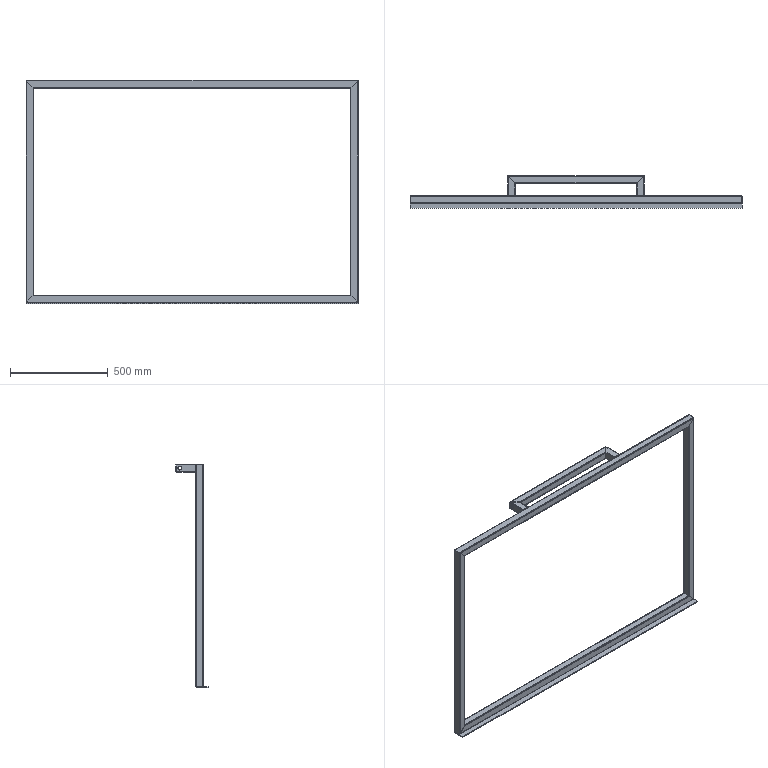Part | STEP file | Stopper rack 12_Default<Machined> | 8 solids | 136 faces | box 1700 x 164 x 1145 mm | volume 2370796 mm3 | plane 76 | cylinder 60 | commonest cylinder face diameters 4 x28 8 x28 20 x4